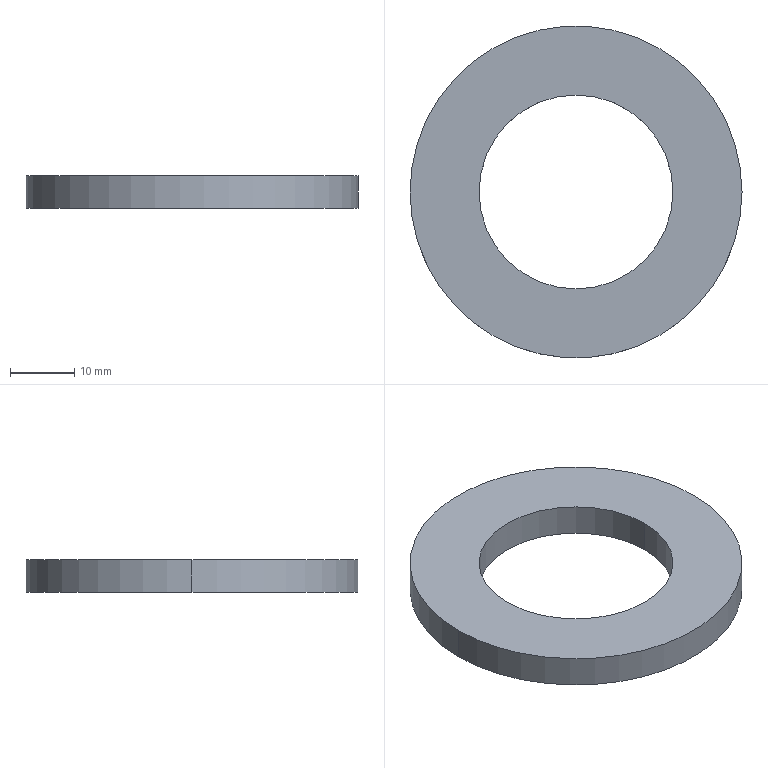Part | SolidWorks | features FlatPattern 1, SMBaseFlange 1, SheetMetal 1 | 1 solid | 6 faces | box 51.7 x 51.7 x 5 mm | volume 6915 mm3 | cylinder 4 | plane 2 | commonest cylinder face diameters 30.2 x2 51.7 x2
STEP:
#1=CARTESIAN_POINT('',(-15.1,0.,5.));
#2=VERTEX_POINT('',#1);
#3=CARTESIAN_POINT('',(15.1,0.,5.));
#4=VERTEX_POINT('',#3);
#5=CARTESIAN_POINT('',(0.,0.,5.));
#6=DIRECTION('',(0.,0.,1.));
#7=DIRECTION('',(1.,0.,0.));
#8=AXIS2_PLACEMENT_3D('',#5,#6,#7);
#9=CIRCLE('',#8,15.1);
#10=EDGE_CURVE('',#2,#4,#9,.T.);
#11=ORIENTED_EDGE('',*,*,#10,.T.);
#12=CARTESIAN_POINT('',(15.1,0.,0.));
#13=VERTEX_POINT('',#12);
#14=CARTESIAN_POINT('',(15.1,0.,5.));
#15=DIRECTION('',(0.,0.,-1.));
#16=VECTOR('',#15,1000.);
#17=LINE('',#14,#16);
#18=EDGE_CURVE('',#4,#13,#17,.T.);
#19=ORIENTED_EDGE('',*,*,#18,.T.);
#20=CARTESIAN_POINT('',(-15.1,0.,0.));
#21=VERTEX_POINT('',#20);
#22=CARTESIAN_POINT('',(0.,0.,0.));
#23=DIRECTION('',(0.,0.,1.));
#24=DIRECTION('',(1.,0.,0.));
#25=AXIS2_PLACEMENT_3D('',#22,#23,#24);
#26=CIRCLE('',#25,15.1);
#27=EDGE_CURVE('',#21,#13,#26,.T.);
#28=ORIENTED_EDGE('',*,*,#27,.F.);
#29=CARTESIAN_POINT('',(-15.1,0.,5.));
#30=DIRECTION('',(0.,0.,-1.));
#31=VECTOR('',#30,1000.);
#32=LINE('',#29,#31);
#33=EDGE_CURVE('',#2,#21,#32,.T.);
#34=ORIENTED_EDGE('',*,*,#33,.F.);
#35=EDGE_LOOP('',(#11,#19,#28,#34));
#36=FACE_OUTER_BOUND('',#35,.T.);
#37=CARTESIAN_POINT('',(0.,0.,5.));
#38=DIRECTION('',(0.,0.,-1.));
#39=DIRECTION('',(-1.,0.,0.));
#40=AXIS2_PLACEMENT_3D('',#37,#38,#39);
#41=CYLINDRICAL_SURFACE('',#40,15.1);
#42=ADVANCED_FACE('',(#36),#41,.F.);
#43=CARTESIAN_POINT('',(25.85,0.,5.));
#44=VERTEX_POINT('',#43);
#45=CARTESIAN_POINT('',(-25.85,0.,5.));
#46=VERTEX_POINT('',#45);
#47=CARTESIAN_POINT('',(0.,0.,5.));
#48=DIRECTION('',(0.,0.,1.));
#49=DIRECTION('',(1.,0.,0.));
#50=AXIS2_PLACEMENT_3D('',#47,#48,#49);
#51=CIRCLE('',#50,25.85);
#52=EDGE_CURVE('',#44,#46,#51,.T.);
#53=ORIENTED_EDGE('',*,*,#52,.F.);
#54=CARTESIAN_POINT('',(25.85,0.,0.));
#55=VERTEX_POINT('',#54);
#56=CARTESIAN_POINT('',(25.85,0.,5.));
#57=DIRECTION('',(0.,0.,-1.));
#58=VECTOR('',#57,1000.);
#59=LINE('',#56,#58);
#60=EDGE_CURVE('',#44,#55,#59,.T.);
#61=ORIENTED_EDGE('',*,*,#60,.T.);
#62=CARTESIAN_POINT('',(-25.85,0.,0.));
#63=VERTEX_POINT('',#62);
#64=CARTESIAN_POINT('',(0.,0.,0.));
#65=DIRECTION('',(0.,0.,1.));
#66=DIRECTION('',(1.,0.,0.));
#67=AXIS2_PLACEMENT_3D('',#64,#65,#66);
#68=CIRCLE('',#67,25.85);
#69=EDGE_CURVE('',#55,#63,#68,.T.);
#70=ORIENTED_EDGE('',*,*,#69,.T.);
#71=CARTESIAN_POINT('',(-25.85,0.,5.));
#72=DIRECTION('',(0.,0.,-1.));
#73=VECTOR('',#72,1000.);
#74=LINE('',#71,#73);
#75=EDGE_CURVE('',#46,#63,#74,.T.);
#76=ORIENTED_EDGE('',*,*,#75,.F.);
#77=EDGE_LOOP('',(#53,#61,#70,#76));
#78=FACE_OUTER_BOUND('',#77,.T.);
#79=CARTESIAN_POINT('',(0.,0.,5.));
#80=DIRECTION('',(0.,0.,-1.));
#81=DIRECTION('',(-1.,0.,0.));
#82=AXIS2_PLACEMENT_3D('',#79,#80,#81);
#83=CYLINDRICAL_SURFACE('',#82,25.85);
#84=ADVANCED_FACE('',(#78),#83,.T.);
#85=CARTESIAN_POINT('',(0.,0.,5.));
#86=DIRECTION('',(0.,0.,1.));
#87=DIRECTION('',(1.,0.,0.));
#88=AXIS2_PLACEMENT_3D('',#85,#86,#87);
#89=CIRCLE('',#88,25.85);
#90=EDGE_CURVE('',#46,#44,#89,.T.);
#91=ORIENTED_EDGE('',*,*,#90,.T.);
#92=ORIENTED_EDGE('',*,*,#52,.T.);
#93=EDGE_LOOP('',(#91,#92));
#94=FACE_OUTER_BOUND('',#93,.T.);
#95=ORIENTED_EDGE('',*,*,#10,.F.);
#96=CARTESIAN_POINT('',(0.,0.,5.));
#97=DIRECTION('',(0.,0.,1.));
#98=DIRECTION('',(1.,0.,0.));
#99=AXIS2_PLACEMENT_3D('',#96,#97,#98);
#100=CIRCLE('',#99,15.1);
#101=EDGE_CURVE('',#4,#2,#100,.T.);
#102=ORIENTED_EDGE('',*,*,#101,.F.);
#103=EDGE_LOOP('',(#95,#102));
#104=FACE_BOUND('',#103,.T.);
#105=CARTESIAN_POINT('',(0.,0.,5.));
#106=DIRECTION('',(0.,0.,1.));
#107=DIRECTION('',(1.,0.,0.));
#108=AXIS2_PLACEMENT_3D('',#105,#106,#107);
#109=PLANE('',#108);
#110=ADVANCED_FACE('',(#94,#104),#109,.T.);
#111=CARTESIAN_POINT('',(0.,0.,0.));
#112=DIRECTION('',(0.,0.,1.));
#113=DIRECTION('',(1.,0.,0.));
#114=AXIS2_PLACEMENT_3D('',#111,#112,#113);
#115=CIRCLE('',#114,25.85);
#116=EDGE_CURVE('',#63,#55,#115,.T.);
#117=ORIENTED_EDGE('',*,*,#116,.F.);
#118=ORIENTED_EDGE('',*,*,#69,.F.);
#119=EDGE_LOOP('',(#117,#118));
#120=FACE_OUTER_BOUND('',#119,.T.);
#121=ORIENTED_EDGE('',*,*,#27,.T.);
#122=CARTESIAN_POINT('',(0.,0.,0.));
#123=DIRECTION('',(0.,0.,1.));
#124=DIRECTION('',(1.,0.,0.));
#125=AXIS2_PLACEMENT_3D('',#122,#123,#124);
#126=CIRCLE('',#125,15.1);
#127=EDGE_CURVE('',#13,#21,#126,.T.);
#128=ORIENTED_EDGE('',*,*,#127,.T.);
#129=EDGE_LOOP('',(#121,#128));
#130=FACE_BOUND('',#129,.T.);
#131=CARTESIAN_POINT('',(0.,0.,0.));
#132=DIRECTION('',(0.,0.,1.));
#133=DIRECTION('',(1.,0.,0.));
#134=AXIS2_PLACEMENT_3D('',#131,#132,#133);
#135=PLANE('',#134);
#136=ADVANCED_FACE('',(#120,#130),#135,.F.);
#137=ORIENTED_EDGE('',*,*,#60,.F.);
#138=ORIENTED_EDGE('',*,*,#90,.F.);
#139=ORIENTED_EDGE('',*,*,#75,.T.);
#140=ORIENTED_EDGE('',*,*,#116,.T.);
#141=EDGE_LOOP('',(#137,#138,#139,#140));
#142=FACE_OUTER_BOUND('',#141,.T.);
#143=CARTESIAN_POINT('',(0.,0.,5.));
#144=DIRECTION('',(0.,0.,-1.));
#145=DIRECTION('',(-1.,0.,0.));
#146=AXIS2_PLACEMENT_3D('',#143,#144,#145);
#147=CYLINDRICAL_SURFACE('',#146,25.85);
#148=ADVANCED_FACE('',(#142),#147,.T.);
#149=ORIENTED_EDGE('',*,*,#18,.F.);
#150=ORIENTED_EDGE('',*,*,#101,.T.);
#151=ORIENTED_EDGE('',*,*,#33,.T.);
#152=ORIENTED_EDGE('',*,*,#127,.F.);
#153=EDGE_LOOP('',(#149,#150,#151,#152));
#154=FACE_OUTER_BOUND('',#153,.T.);
#155=CARTESIAN_POINT('',(0.,0.,5.));
#156=DIRECTION('',(0.,0.,-1.));
#157=DIRECTION('',(-1.,0.,0.));
#158=AXIS2_PLACEMENT_3D('',#155,#156,#157);
#159=CYLINDRICAL_SURFACE('',#158,15.1);
#160=ADVANCED_FACE('',(#154),#159,.F.);
#161=CLOSED_SHELL('',(#42,#84,#110,#136,#148,#160));
#162=MANIFOLD_SOLID_BREP('',#161);
#163=CARTESIAN_POINT('',(0.,0.,0.));
#164=DIRECTION('',(0.,0.,1.));
#165=DIRECTION('',(1.,0.,0.));
#166=AXIS2_PLACEMENT_3D('',#163,#164,#165);
#167=(LENGTH_UNIT()NAMED_UNIT(*)SI_UNIT(.MILLI.,.METRE.));
#168=UNCERTAINTY_MEASURE_WITH_UNIT(LENGTH_MEASURE(0.00001),#167,'','');
#169=(NAMED_UNIT(*)PLANE_ANGLE_UNIT()SI_UNIT($,.RADIAN.));
#170=(NAMED_UNIT(*)SI_UNIT($,.STERADIAN.)SOLID_ANGLE_UNIT());
#171=(GEOMETRIC_REPRESENTATION_CONTEXT(3)GLOBAL_UNCERTAINTY_ASSIGNED_CONTEXT((#168))GLOBAL_UNIT_ASSIGNED_CONTEXT((#167,#169,#170))REPRESENTATION_CONTEXT('',''));
#172=ADVANCED_BREP_SHAPE_REPRESENTATION('',(#162,#166),#171);